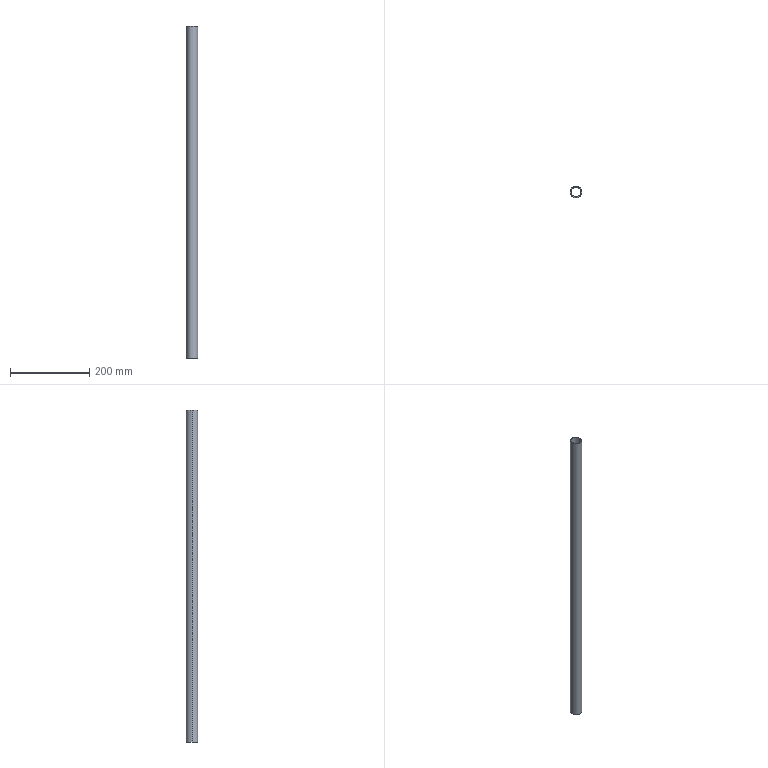Part | SolidWorks | features Extrusion 1 | 1 solid | 6 faces | box 28.9 x 28.9 x 840 mm | volume 105036 mm3 | cylinder 4 | plane 2 | commonest cylinder face diameters 26 x2 28.9 x2
STEP:
#1=CARTESIAN_POINT('',(-13.,0.,840.));
#2=VERTEX_POINT('',#1);
#3=CARTESIAN_POINT('',(13.,0.,840.));
#4=VERTEX_POINT('',#3);
#5=CARTESIAN_POINT('',(0.,0.,840.));
#6=DIRECTION('',(0.,0.,1.));
#7=DIRECTION('',(1.,0.,0.));
#8=AXIS2_PLACEMENT_3D('',#5,#6,#7);
#9=CIRCLE('',#8,13.);
#10=EDGE_CURVE('',#2,#4,#9,.T.);
#11=ORIENTED_EDGE('',*,*,#10,.T.);
#12=CARTESIAN_POINT('',(13.,0.,0.));
#13=VERTEX_POINT('',#12);
#14=CARTESIAN_POINT('',(13.,0.,840.));
#15=DIRECTION('',(0.,0.,-1.));
#16=VECTOR('',#15,1000.);
#17=LINE('',#14,#16);
#18=EDGE_CURVE('',#4,#13,#17,.T.);
#19=ORIENTED_EDGE('',*,*,#18,.T.);
#20=CARTESIAN_POINT('',(-13.,0.,0.));
#21=VERTEX_POINT('',#20);
#22=CARTESIAN_POINT('',(0.,0.,0.));
#23=DIRECTION('',(0.,0.,1.));
#24=DIRECTION('',(1.,0.,0.));
#25=AXIS2_PLACEMENT_3D('',#22,#23,#24);
#26=CIRCLE('',#25,13.);
#27=EDGE_CURVE('',#21,#13,#26,.T.);
#28=ORIENTED_EDGE('',*,*,#27,.F.);
#29=CARTESIAN_POINT('',(-13.,0.,840.));
#30=DIRECTION('',(0.,0.,-1.));
#31=VECTOR('',#30,1000.);
#32=LINE('',#29,#31);
#33=EDGE_CURVE('',#2,#21,#32,.T.);
#34=ORIENTED_EDGE('',*,*,#33,.F.);
#35=EDGE_LOOP('',(#11,#19,#28,#34));
#36=FACE_OUTER_BOUND('',#35,.T.);
#37=CARTESIAN_POINT('',(0.,0.,840.));
#38=DIRECTION('',(0.,0.,-1.));
#39=DIRECTION('',(-1.,0.,0.));
#40=AXIS2_PLACEMENT_3D('',#37,#38,#39);
#41=CYLINDRICAL_SURFACE('',#40,13.);
#42=ADVANCED_FACE('',(#36),#41,.F.);
#43=CARTESIAN_POINT('',(14.45,0.,840.));
#44=VERTEX_POINT('',#43);
#45=CARTESIAN_POINT('',(-14.45,0.,840.));
#46=VERTEX_POINT('',#45);
#47=CARTESIAN_POINT('',(0.,0.,840.));
#48=DIRECTION('',(0.,0.,1.));
#49=DIRECTION('',(1.,0.,0.));
#50=AXIS2_PLACEMENT_3D('',#47,#48,#49);
#51=CIRCLE('',#50,14.45);
#52=EDGE_CURVE('',#44,#46,#51,.T.);
#53=ORIENTED_EDGE('',*,*,#52,.F.);
#54=CARTESIAN_POINT('',(14.45,0.,0.));
#55=VERTEX_POINT('',#54);
#56=CARTESIAN_POINT('',(14.45,0.,840.));
#57=DIRECTION('',(0.,0.,-1.));
#58=VECTOR('',#57,1000.);
#59=LINE('',#56,#58);
#60=EDGE_CURVE('',#44,#55,#59,.T.);
#61=ORIENTED_EDGE('',*,*,#60,.T.);
#62=CARTESIAN_POINT('',(-14.45,0.,0.));
#63=VERTEX_POINT('',#62);
#64=CARTESIAN_POINT('',(0.,0.,0.));
#65=DIRECTION('',(0.,0.,1.));
#66=DIRECTION('',(1.,0.,0.));
#67=AXIS2_PLACEMENT_3D('',#64,#65,#66);
#68=CIRCLE('',#67,14.45);
#69=EDGE_CURVE('',#55,#63,#68,.T.);
#70=ORIENTED_EDGE('',*,*,#69,.T.);
#71=CARTESIAN_POINT('',(-14.45,0.,840.));
#72=DIRECTION('',(0.,0.,-1.));
#73=VECTOR('',#72,1000.);
#74=LINE('',#71,#73);
#75=EDGE_CURVE('',#46,#63,#74,.T.);
#76=ORIENTED_EDGE('',*,*,#75,.F.);
#77=EDGE_LOOP('',(#53,#61,#70,#76));
#78=FACE_OUTER_BOUND('',#77,.T.);
#79=CARTESIAN_POINT('',(0.,0.,840.));
#80=DIRECTION('',(0.,0.,-1.));
#81=DIRECTION('',(-1.,0.,0.));
#82=AXIS2_PLACEMENT_3D('',#79,#80,#81);
#83=CYLINDRICAL_SURFACE('',#82,14.45);
#84=ADVANCED_FACE('',(#78),#83,.T.);
#85=CARTESIAN_POINT('',(0.,0.,840.));
#86=DIRECTION('',(0.,0.,1.));
#87=DIRECTION('',(1.,0.,0.));
#88=AXIS2_PLACEMENT_3D('',#85,#86,#87);
#89=CIRCLE('',#88,14.45);
#90=EDGE_CURVE('',#46,#44,#89,.T.);
#91=ORIENTED_EDGE('',*,*,#90,.T.);
#92=ORIENTED_EDGE('',*,*,#52,.T.);
#93=EDGE_LOOP('',(#91,#92));
#94=FACE_OUTER_BOUND('',#93,.T.);
#95=ORIENTED_EDGE('',*,*,#10,.F.);
#96=CARTESIAN_POINT('',(0.,0.,840.));
#97=DIRECTION('',(0.,0.,1.));
#98=DIRECTION('',(1.,0.,0.));
#99=AXIS2_PLACEMENT_3D('',#96,#97,#98);
#100=CIRCLE('',#99,13.);
#101=EDGE_CURVE('',#4,#2,#100,.T.);
#102=ORIENTED_EDGE('',*,*,#101,.F.);
#103=EDGE_LOOP('',(#95,#102));
#104=FACE_BOUND('',#103,.T.);
#105=CARTESIAN_POINT('',(0.,0.,840.));
#106=DIRECTION('',(0.,0.,1.));
#107=DIRECTION('',(1.,0.,0.));
#108=AXIS2_PLACEMENT_3D('',#105,#106,#107);
#109=PLANE('',#108);
#110=ADVANCED_FACE('',(#94,#104),#109,.T.);
#111=CARTESIAN_POINT('',(0.,0.,0.));
#112=DIRECTION('',(0.,0.,1.));
#113=DIRECTION('',(1.,0.,0.));
#114=AXIS2_PLACEMENT_3D('',#111,#112,#113);
#115=CIRCLE('',#114,14.45);
#116=EDGE_CURVE('',#63,#55,#115,.T.);
#117=ORIENTED_EDGE('',*,*,#116,.F.);
#118=ORIENTED_EDGE('',*,*,#69,.F.);
#119=EDGE_LOOP('',(#117,#118));
#120=FACE_OUTER_BOUND('',#119,.T.);
#121=ORIENTED_EDGE('',*,*,#27,.T.);
#122=CARTESIAN_POINT('',(0.,0.,0.));
#123=DIRECTION('',(0.,0.,1.));
#124=DIRECTION('',(1.,0.,0.));
#125=AXIS2_PLACEMENT_3D('',#122,#123,#124);
#126=CIRCLE('',#125,13.);
#127=EDGE_CURVE('',#13,#21,#126,.T.);
#128=ORIENTED_EDGE('',*,*,#127,.T.);
#129=EDGE_LOOP('',(#121,#128));
#130=FACE_BOUND('',#129,.T.);
#131=CARTESIAN_POINT('',(0.,0.,0.));
#132=DIRECTION('',(0.,0.,1.));
#133=DIRECTION('',(1.,0.,0.));
#134=AXIS2_PLACEMENT_3D('',#131,#132,#133);
#135=PLANE('',#134);
#136=ADVANCED_FACE('',(#120,#130),#135,.F.);
#137=ORIENTED_EDGE('',*,*,#60,.F.);
#138=ORIENTED_EDGE('',*,*,#90,.F.);
#139=ORIENTED_EDGE('',*,*,#75,.T.);
#140=ORIENTED_EDGE('',*,*,#116,.T.);
#141=EDGE_LOOP('',(#137,#138,#139,#140));
#142=FACE_OUTER_BOUND('',#141,.T.);
#143=CARTESIAN_POINT('',(0.,0.,840.));
#144=DIRECTION('',(0.,0.,-1.));
#145=DIRECTION('',(-1.,0.,0.));
#146=AXIS2_PLACEMENT_3D('',#143,#144,#145);
#147=CYLINDRICAL_SURFACE('',#146,14.45);
#148=ADVANCED_FACE('',(#142),#147,.T.);
#149=ORIENTED_EDGE('',*,*,#18,.F.);
#150=ORIENTED_EDGE('',*,*,#101,.T.);
#151=ORIENTED_EDGE('',*,*,#33,.T.);
#152=ORIENTED_EDGE('',*,*,#127,.F.);
#153=EDGE_LOOP('',(#149,#150,#151,#152));
#154=FACE_OUTER_BOUND('',#153,.T.);
#155=CARTESIAN_POINT('',(0.,0.,840.));
#156=DIRECTION('',(0.,0.,-1.));
#157=DIRECTION('',(-1.,0.,0.));
#158=AXIS2_PLACEMENT_3D('',#155,#156,#157);
#159=CYLINDRICAL_SURFACE('',#158,13.);
#160=ADVANCED_FACE('',(#154),#159,.F.);
#161=CLOSED_SHELL('',(#42,#84,#110,#136,#148,#160));
#162=MANIFOLD_SOLID_BREP('',#161);
#163=CARTESIAN_POINT('',(0.,0.,0.));
#164=DIRECTION('',(0.,0.,1.));
#165=DIRECTION('',(1.,0.,0.));
#166=AXIS2_PLACEMENT_3D('',#163,#164,#165);
#167=(LENGTH_UNIT()NAMED_UNIT(*)SI_UNIT(.MILLI.,.METRE.));
#168=UNCERTAINTY_MEASURE_WITH_UNIT(LENGTH_MEASURE(0.00001),#167,'','');
#169=(NAMED_UNIT(*)PLANE_ANGLE_UNIT()SI_UNIT($,.RADIAN.));
#170=(NAMED_UNIT(*)SI_UNIT($,.STERADIAN.)SOLID_ANGLE_UNIT());
#171=(GEOMETRIC_REPRESENTATION_CONTEXT(3)GLOBAL_UNCERTAINTY_ASSIGNED_CONTEXT((#168))GLOBAL_UNIT_ASSIGNED_CONTEXT((#167,#169,#170))REPRESENTATION_CONTEXT('',''));
#172=ADVANCED_BREP_SHAPE_REPRESENTATION('',(#162,#166),#171);